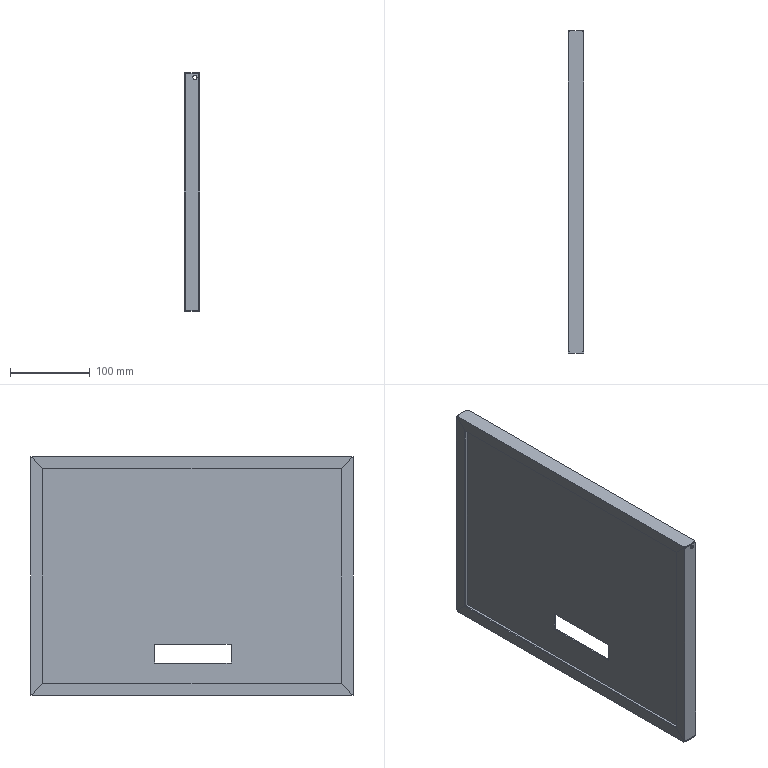Part | 1 solid | 78 faces | box 19.5 x 405 x 300 mm | volume 243866 mm3 | plane 74 | cylinder 4 | commonest cylinder face diameters 5.2 x4